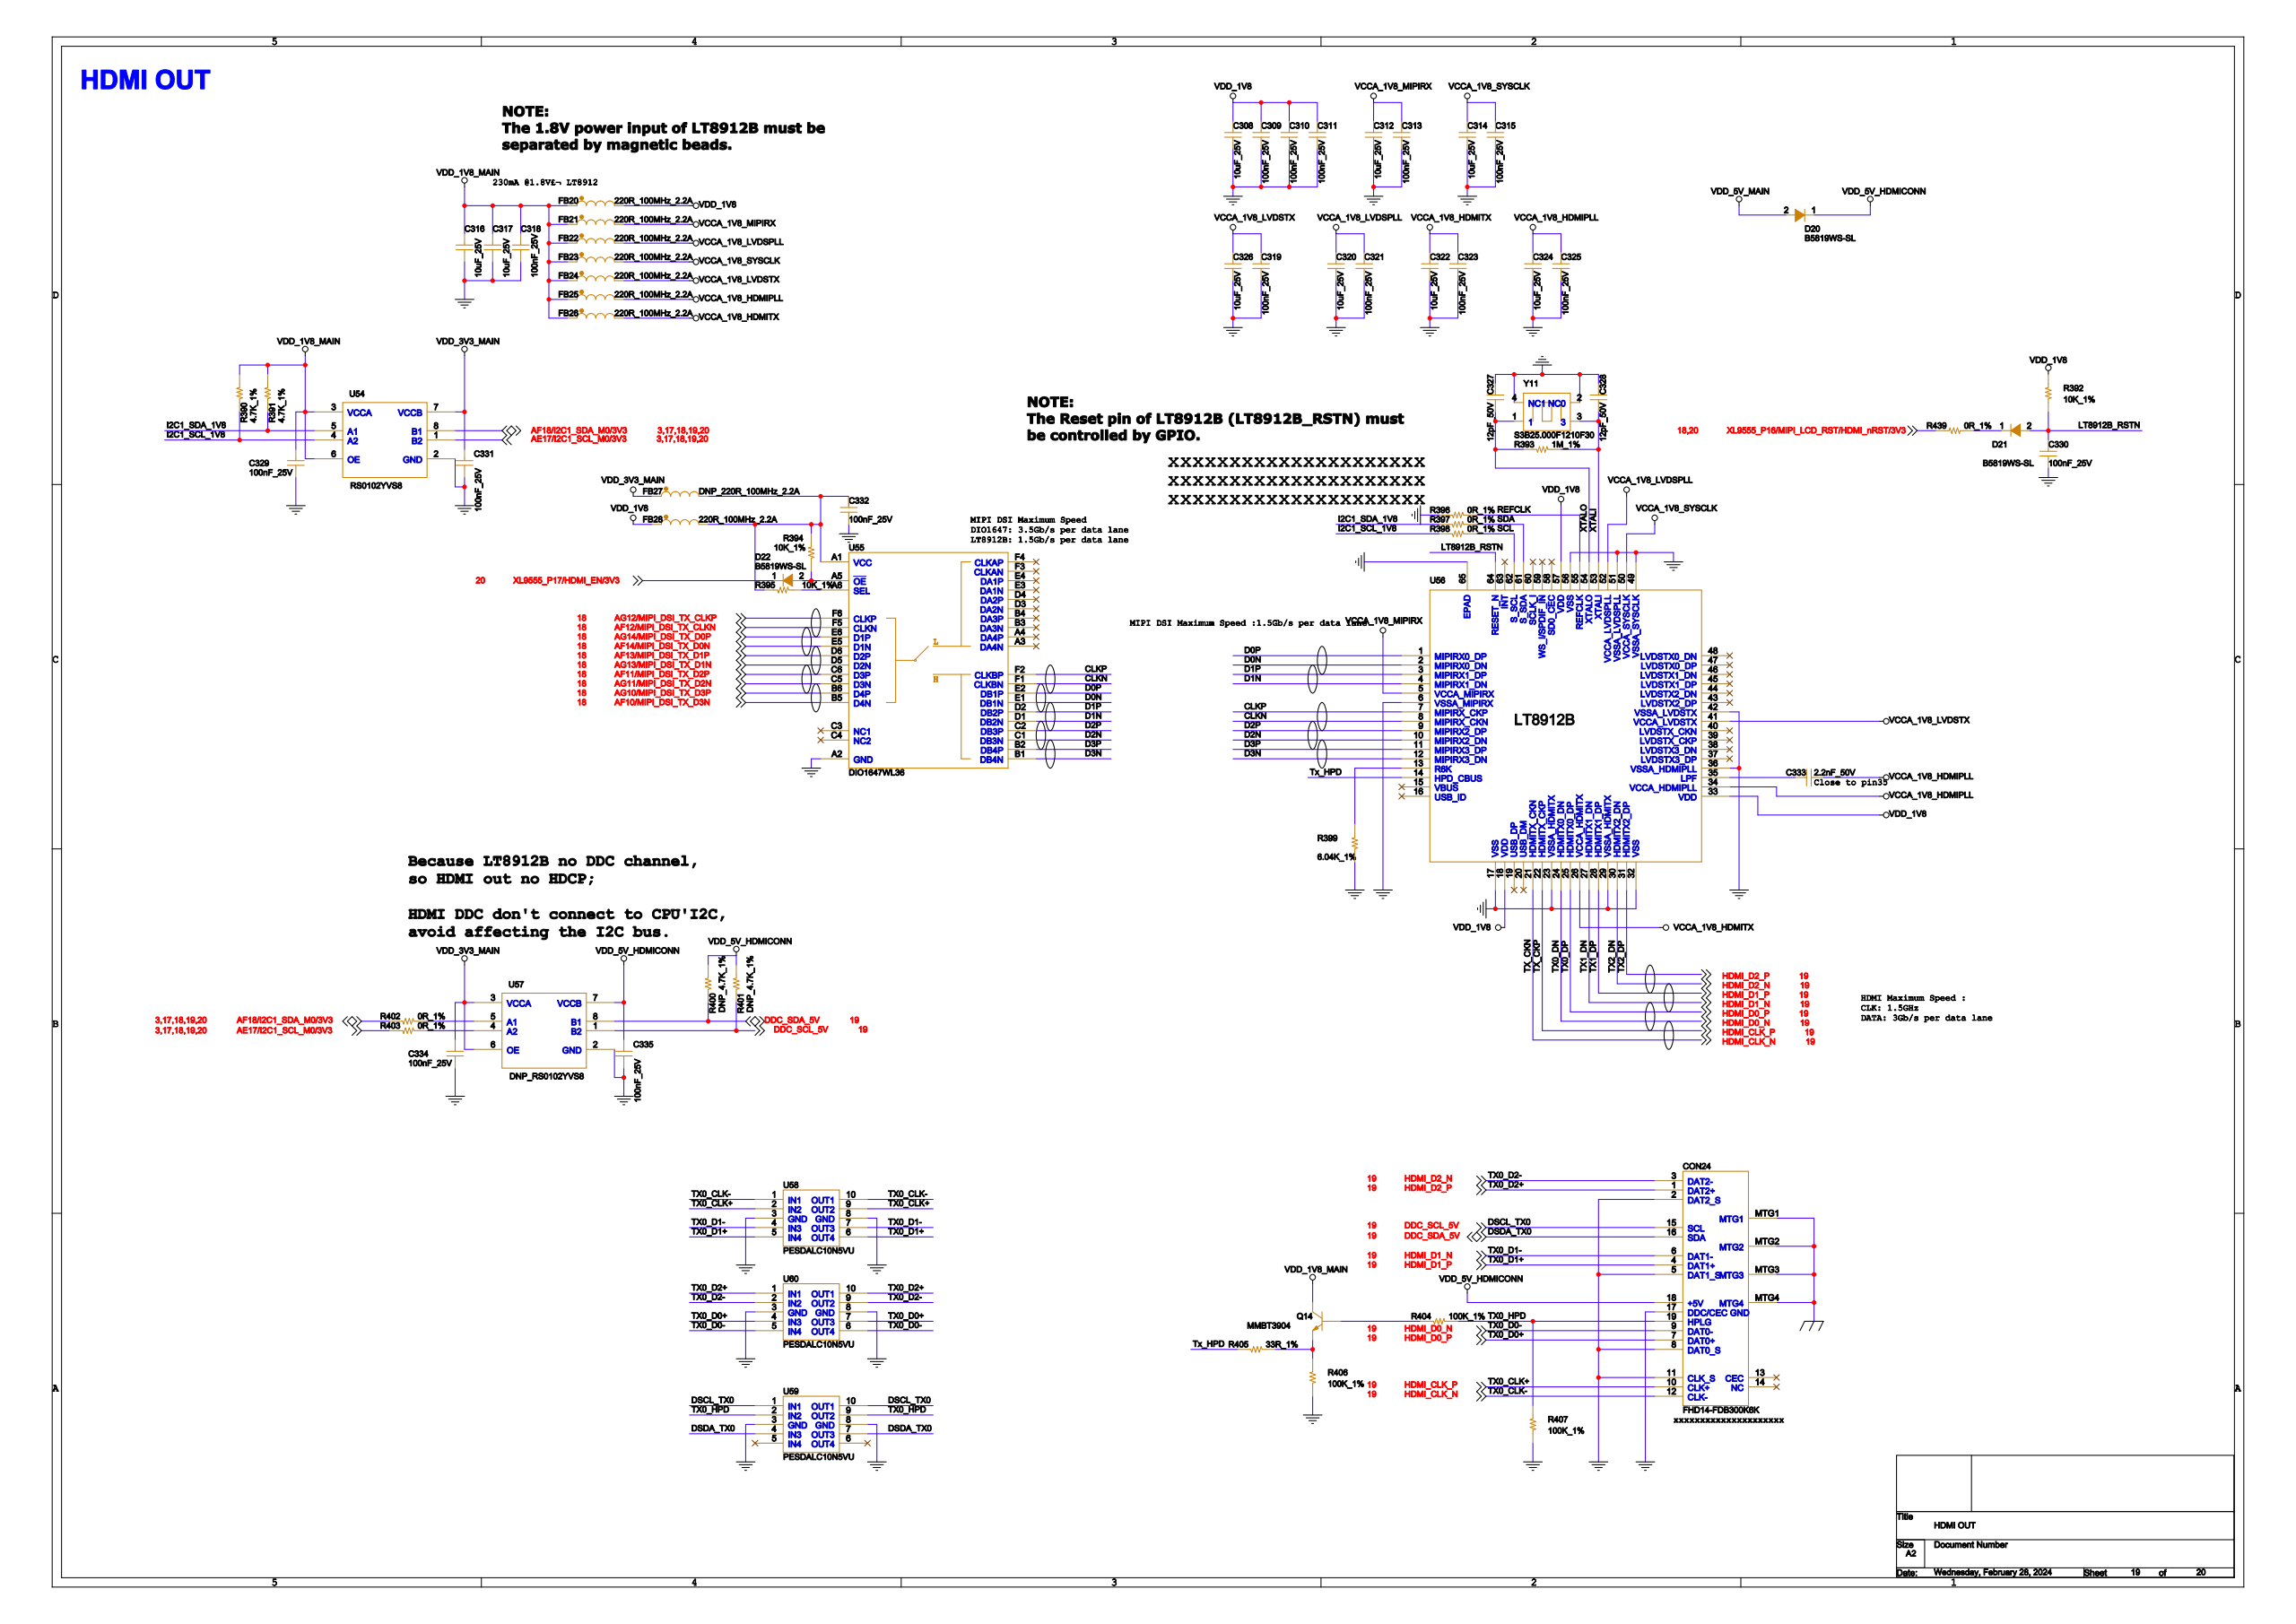Circuit board | Cadence Allegro | 1024 parts | 682 nets | one sheet of the schematic
Parts on this sheet (reference | value | footprint):
C308 | 10uF_25V | C0603
C309 | 100nF_25V | C0402
C310 | 100nF_25V | C0402
C311 | 100nF_25V | C0402
C312 | 10uF_25V | C0603
C313 | 100nF_25V | C0402
C314 | 10uF_25V | C0603
C315 | 100nF_25V | C0402
C319 | 100nF_25V | C0402
C320 | 10uF_25V | C0603
C321 | 100nF_25V | C0402
C322 | 10uF_25V | C0603
C323 | 100nF_25V | C0402
C324 | 10uF_25V | C0603
C325 | 100nF_25V | C0402
C326 | 10uF_25V | C0603
C327 | 12pF_50V | C0402
C328 | 12pF_50V | C0402
C329 | 100nF_25V | C0402
C330 | 100nF_25V | C0402
C331 | 100nF_25V | C0402
C332 | 100nF_25V | C0402
C333 | 2.2nF_50V | C0603
C334 | 100nF_25V | C0402
C335 | 100nF_25V | C0402
CON24 | FHD14-FDB300K6K | DIP_HDMI-A
D20 | B5819WS-SL | SOD-323
D21 | B5819WS-SL | SOD-323
D22 | B5819WS-SL | SOD-323
FB20 | 220R_100MHz_2A | L0603
FB21 | 220R_100MHz_2A | L0603
FB22 | 220R_100MHz_2A | L0603
FB23 | 220R_100MHz_2A | L0603
FB24 | 220R_100MHz_2A | L0603
FB25 | 220R_100MHz_2A | L0603
FB26 | 220R_100MHz_2A | L0603
FB27 | DNP_220R_100MHz_2A | L0603
FB28 | 220R_100MHz_2A | L0603
Q14 | MMBT3904 | SOT23-3_DBZ3
R390 | 4.7K_1% | R0402
R391 | 4.7K_1% | R0402
R392 | 10K_1% | R0402
R393 | 1M_1% | R0603
R394 | 10K_1% | R0402
R395 | 10K_1% | R0402
R396 | 0R_1% | R0402
R397 | 0R_1% | R0402
R398 | 0R_1% | R0402
R399 | 6.04K_1% | R0402
R400 | DNP_4.7K_1% | R0402
R401 | DNP_4.7K_1% | R0402
R402 | 0R_1% | R0402
R403 | 0R_1% | R0402
R404 | 100K_1% | R0402
R405 | 33R_1% | R0402
R406 | 100K_1% | R0402
R407 | 100K_1% | R0402
R439 | 0R_1% | R0402
U54 | RS0102YVS8 | SOP8-20-91
U55 | DIO1647 | WLCSP-36-0D4MM
U56 | LT8912B | QFN64_LT8912B
U57 | DNP_RS0102YVS8 | SOP8-20-91
U58 | PESDALC10N5VU | DFN-10-2510
U59 | PESDALC10N5VU | DFN-10-2510
U60 | PESDALC10N5VU | DFN-10-2510
Y11 | S3B25.000F1210F30 | SMD_3225
Nets of these parts (net: part-pin ...):
GND: C308-2 C309-2 C310-2 C311-2 C312-2 C313-2 C314-2 C315-2 C319-2 C320-2 C321-2 C322-2 C323-2 C324-2 C325-2 C326-2 C327-1 C328-1 C329-2 C330-2 C331-2 C332-2 C334-2 C335-2 R396-1 R399-1 R406-1 R407-1 U54-2 U57-2 U58-3 U58-8 U59-3 U59-8 U60-3 U60-8 Y11-2 Y11-4 CON24-2 CON24-5 CON24-8 CON24-11 CON24-17 U55-A2 U56-6 U56-17 U56-23 U56-29 U56-32 U56-36 U56-42 U56-49 U56-51 U56-56 U56-65
VDD_5V_MAIN: D20-2
VDD_1V8_MAIN: C329-1 FB20-1 FB21-1 FB22-1 FB23-1 FB24-1 FB25-1 FB26-1 Q14-3 R390-2 R391-2 U54-3 U54-6
VDD_3V3_MAIN: C331-1 C334-1 FB27-1 U54-7 U57-3 U57-6
VDD_5V_HDMICONN: C335-1 D20-1 R400-2 R401-2 U57-7 CON24-18
HDMI_CLK_P: U58-2 U58-9 CON24-10 U56-22
HDMI_CLK_N: U58-1 U58-10 CON24-12 U56-21
HDMI_D0_P: U60-4 U60-7 CON24-7 U56-25
HDMI_D0_N: U60-5 U60-6 CON24-9 U56-24
HDMI_D1_P: U58-5 U58-6 CON24-4 U56-28
HDMI_D1_N: U58-4 U58-7 CON24-6 U56-27
HDMI_D2_P: U60-1 U60-10 CON24-1 U56-31
HDMI_D2_N: U60-2 U60-9 CON24-3 U56-30
TX0_HPD: R404-1 R407-2 U59-2 U59-9 CON24-19
DDC_SCL_5V: R401-1 U57-1 U59-1 U59-10 CON24-15
DDC_SDA_5V: R400-1 U57-8 U59-4 U59-7 CON24-16
VDD_1V8: C308-1 C309-1 C310-1 C311-1 FB20-2 FB28-1 R392-2 U56-18 U56-33 U56-57
VCCA_1V8_MIPIRX: C312-1 C313-1 FB21-2 U56-5
VCCA_1V8_SYSCLK: C314-1 C315-1 FB23-2 U56-50
VCCA_1V8_LVDSPLL: C320-1 C321-1 FB22-2 U56-52
VCCA_1V8_HDMITX: C322-1 C323-1 FB26-2 U56-26
VCCA_1V8_HDMIPLL: C324-1 C325-1 C333-2 FB25-2 U56-34
VCCA_1V8_LVDSTX: C319-1 C326-1 FB24-2 U56-41
LT8912B_RSTN: C330-1 D21-2 R392-1 U56-64
XTALO: C327-2 R393-2 Y11-1 U56-54
XTALI: C328-2 R393-1 Y11-3 U56-53
N21893217: C332-1 FB27-2 FB28-2 R394-1 R395-1 U55-A1
N21638199: C333-1 U56-35
AF18/I2C1_SDA_M0/3V3: R402-2 U54-8
AE17/I2C1_SCL_M0/3V3: R403-2 U54-1
N22247543: D21-1 R439-1
XL9555_P17/HDMI_EN/3V3: D22-1
N21893228: D22-2 R394-2 U55-A5
I2C1_SCL_1V8: R390-1 R398-1 U54-4
I2C1_SDA_1V8: R391-1 R397-1 U54-5
N21640508: Q14-1 R404-2
N21640498: Q14-2 R405-1 R406-2
N21893329: R395-2 U55-A6
N21637999: R399-2 U56-13
CLKN: U55-F1 U56-8
CLKP: U55-F2 U56-7
AF12/MIPI_DSI_TX_CLKN: U55-F5
AG12/MIPI_DSI_TX_CLKP: U55-F6
AF14/MIPI_DSI_TX_D0N: U55-E5
AG14/MIPI_DSI_TX_D0P: U55-E6
AG13/MIPI_DSI_TX_D1N: U55-D5
AF13/MIPI_DSI_TX_D1P: U55-D6
AG11/MIPI_DSI_TX_D2N: U55-C5
AF11/MIPI_DSI_TX_D2P: U55-C6
AF10/MIPI_DSI_TX_D3N: U55-B5
AG10/MIPI_DSI_TX_D3P: U55-B6
D0N: U55-E1 U56-2
D0P: U55-E2 U56-1
D1N: U55-D1 U56-4
D1P: U55-D2 U56-3
D2N: U55-C1 U56-10
D2P: U55-C2 U56-9
D3N: U55-B1 U56-12
D3P: U55-B2 U56-11
TX_HPD: R405-2 U56-14
REFCLK: R396-2 U56-55
SCL: R398-2 U56-62
SDA: R397-2 U56-61
N21898964: R402-1 U57-5
N21898967: R403-1 U57-4
XL9555_P16/MIPI_LCD_RST/HDMI_NR: R439-2